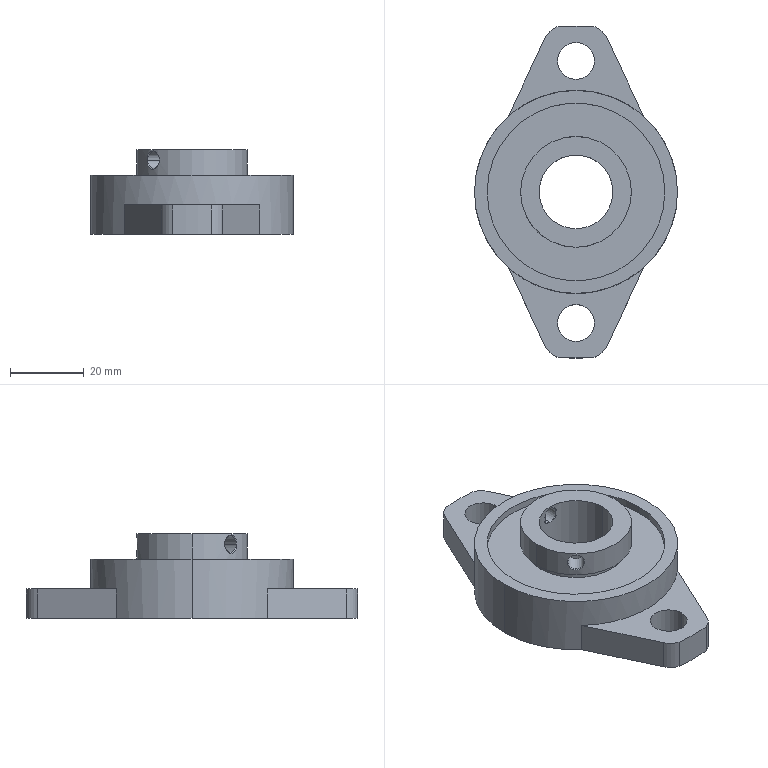Part | STEP file | HBT20_HBT20 | 1 solid | 53 faces | box 55 x 90 x 23 mm | volume 35795 mm3 | cylinder 26 | plane 17 | cone 8 | torus 2 | commonest cylinder face diameters 4.459 x4 10 x4 11 x4 48.125 x4 20 x2 26.875 x2